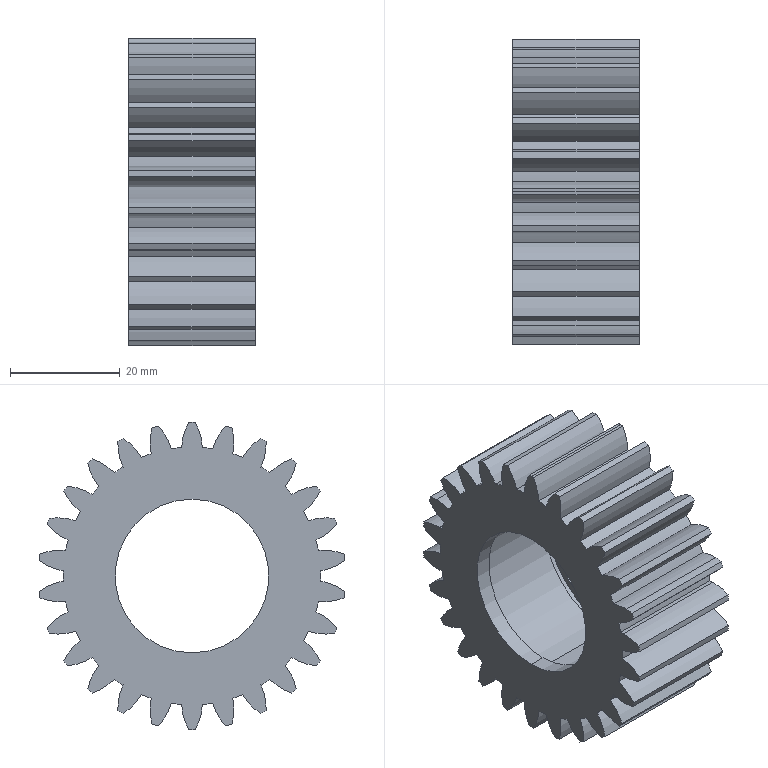Part | SolidWorks | features ICE 26, RevCut 1, Revolution 1 | 1 solid | 122 faces | box 23 x 55.72 x 56 mm | volume 29460 mm3 | cylinder 117 | plane 5 | commonest cylinder face diameters 20.8 x56 56 x27 46.998 x26 32 x4 28 x2 34.5 x2